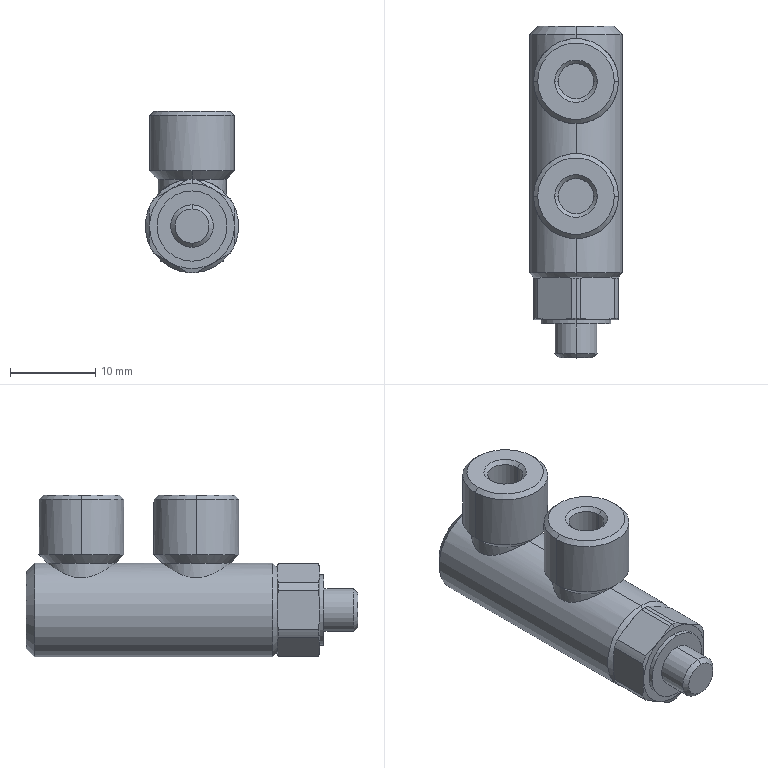Part | SolidWorks | features BaseBody 1 | 1 solid | 73 faces | box 11 x 39 x 19 mm | volume 4357 mm3 | cone 32 | cylinder 27 | plane 14 | commonest cylinder face diameters 11 x9 8 x6 4.134 x4 10 x4 5 x2 8.25 x2